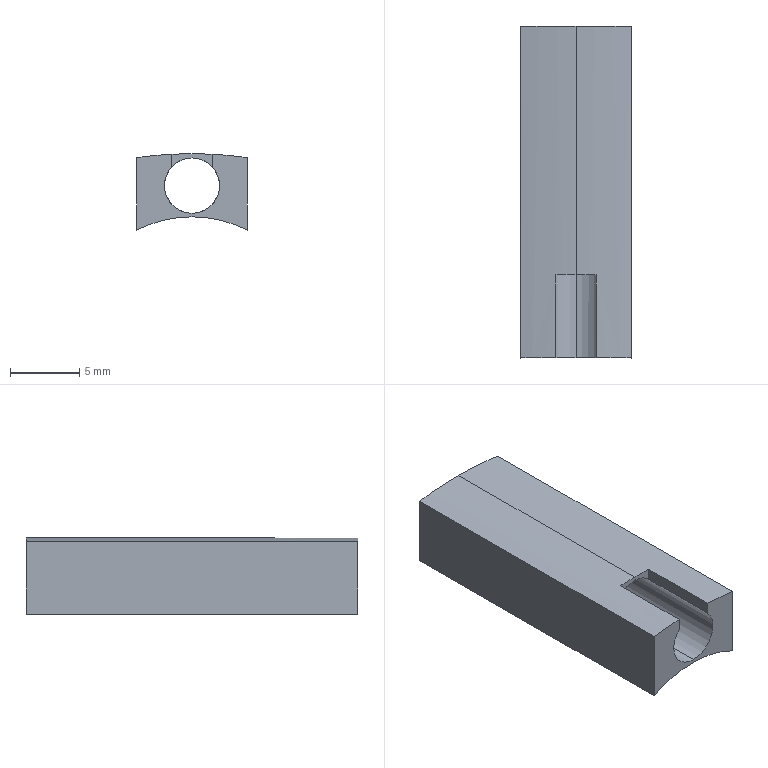Part | NX | 1 solid | 13 faces | box 8 x 24 x 5.527 mm | volume 608.204 mm3 | plane 7 | cylinder 6 | commonest cylinder face diameters 4 x2 17.5 x2 58 x2
STEP:
#1=CARTESIAN_POINT('',(0.,12.,-1.4));
#2=VERTEX_POINT('',#1);
#3=CARTESIAN_POINT('',(0.,12.,2.6));
#4=VERTEX_POINT('',#3);
#5=CARTESIAN_POINT('',(0.,12.,0.6));
#6=DIRECTION('',(0.,1.,0.));
#7=DIRECTION('',(0.,0.,1.));
#8=AXIS2_PLACEMENT_3D('',#5,#6,#7);
#9=CIRCLE('',#8,2.);
#10=EDGE_CURVE('',#2,#4,#9,.T.);
#11=ORIENTED_EDGE('',*,*,#10,.T.);
#12=CARTESIAN_POINT('',(0.,-6.,2.6));
#13=VERTEX_POINT('',#12);
#14=CARTESIAN_POINT('',(0.,-12.,2.6));
#15=DIRECTION('',(0.,1.,0.));
#16=VECTOR('',#15,1000.);
#17=LINE('',#14,#16);
#18=EDGE_CURVE('',#13,#4,#17,.T.);
#19=ORIENTED_EDGE('',*,*,#18,.F.);
#20=CARTESIAN_POINT('',(-1.45,-6.,1.977));
#21=VERTEX_POINT('',#20);
#22=CARTESIAN_POINT('',(0.,-6.,0.6));
#23=DIRECTION('',(0.,1.,0.));
#24=DIRECTION('',(0.,0.,-1.));
#25=AXIS2_PLACEMENT_3D('',#22,#23,#24);
#26=CIRCLE('',#25,2.);
#27=EDGE_CURVE('',#21,#13,#26,.T.);
#28=ORIENTED_EDGE('',*,*,#27,.F.);
#29=CARTESIAN_POINT('',(-1.45,-12.,1.977));
#30=VERTEX_POINT('',#29);
#31=CARTESIAN_POINT('',(-1.45,-6.,1.977));
#32=DIRECTION('',(0.,-1.,0.));
#33=VECTOR('',#32,1000.);
#34=LINE('',#31,#33);
#35=EDGE_CURVE('',#21,#30,#34,.T.);
#36=ORIENTED_EDGE('',*,*,#35,.T.);
#37=CARTESIAN_POINT('',(0.,-12.,-1.4));
#38=VERTEX_POINT('',#37);
#39=CARTESIAN_POINT('',(0.,-12.,0.6));
#40=DIRECTION('',(0.,1.,0.));
#41=DIRECTION('',(0.,0.,1.));
#42=AXIS2_PLACEMENT_3D('',#39,#40,#41);
#43=CIRCLE('',#42,2.);
#44=EDGE_CURVE('',#38,#30,#43,.T.);
#45=ORIENTED_EDGE('',*,*,#44,.F.);
#46=CARTESIAN_POINT('',(0.,-12.,-1.4));
#47=DIRECTION('',(0.,1.,0.));
#48=VECTOR('',#47,1000.);
#49=LINE('',#46,#48);
#50=EDGE_CURVE('',#38,#2,#49,.T.);
#51=ORIENTED_EDGE('',*,*,#50,.T.);
#52=EDGE_LOOP('',(#11,#19,#28,#36,#45,#51));
#53=FACE_BOUND('',#52,.T.);
#54=CARTESIAN_POINT('',(0.,-12.,0.6));
#55=DIRECTION('',(0.,1.,0.));
#56=DIRECTION('',(0.,0.,1.));
#57=AXIS2_PLACEMENT_3D('',#54,#55,#56);
#58=CYLINDRICAL_SURFACE('',#57,2.);
#59=ADVANCED_FACE('',(#53),#58,.F.);
#60=CARTESIAN_POINT('',(0.,-12.,-1.657));
#61=VERTEX_POINT('',#60);
#62=CARTESIAN_POINT('',(0.,12.,-1.657));
#63=VERTEX_POINT('',#62);
#64=CARTESIAN_POINT('',(0.,-12.,-1.657));
#65=DIRECTION('',(0.,1.,0.));
#66=VECTOR('',#65,1000.);
#67=LINE('',#64,#66);
#68=EDGE_CURVE('',#61,#63,#67,.T.);
#69=ORIENTED_EDGE('',*,*,#68,.F.);
#70=CARTESIAN_POINT('',(-4.,-12.,-2.625));
#71=VERTEX_POINT('',#70);
#72=CARTESIAN_POINT('',(0.,-12.,-10.407));
#73=DIRECTION('',(0.,-1.,0.));
#74=DIRECTION('',(0.,0.,1.));
#75=AXIS2_PLACEMENT_3D('',#72,#73,#74);
#76=CIRCLE('',#75,8.75);
#77=EDGE_CURVE('',#61,#71,#76,.T.);
#78=ORIENTED_EDGE('',*,*,#77,.T.);
#79=CARTESIAN_POINT('',(-4.,12.,-2.625));
#80=VERTEX_POINT('',#79);
#81=CARTESIAN_POINT('',(-4.,-12.,-2.625));
#82=DIRECTION('',(0.,1.,0.));
#83=VECTOR('',#82,1000.);
#84=LINE('',#81,#83);
#85=EDGE_CURVE('',#71,#80,#84,.T.);
#86=ORIENTED_EDGE('',*,*,#85,.T.);
#87=CARTESIAN_POINT('',(0.,12.,-10.407));
#88=DIRECTION('',(0.,-1.,0.));
#89=DIRECTION('',(0.,0.,1.));
#90=AXIS2_PLACEMENT_3D('',#87,#88,#89);
#91=CIRCLE('',#90,8.75);
#92=EDGE_CURVE('',#63,#80,#91,.T.);
#93=ORIENTED_EDGE('',*,*,#92,.F.);
#94=EDGE_LOOP('',(#69,#78,#86,#93));
#95=FACE_BOUND('',#94,.T.);
#96=CARTESIAN_POINT('',(0.,-12.,-10.407));
#97=DIRECTION('',(0.,1.,0.));
#98=DIRECTION('',(0.,0.,1.));
#99=AXIS2_PLACEMENT_3D('',#96,#97,#98);
#100=CYLINDRICAL_SURFACE('',#99,8.75);
#101=ADVANCED_FACE('',(#95),#100,.F.);
#102=CARTESIAN_POINT('',(0.,-6.,2.902));
#103=VERTEX_POINT('',#102);
#104=CARTESIAN_POINT('',(0.,12.,2.902));
#105=VERTEX_POINT('',#104);
#106=CARTESIAN_POINT('',(0.,-12.,2.902));
#107=DIRECTION('',(0.,1.,0.));
#108=VECTOR('',#107,1000.);
#109=LINE('',#106,#108);
#110=EDGE_CURVE('',#103,#105,#109,.T.);
#111=ORIENTED_EDGE('',*,*,#110,.F.);
#112=CARTESIAN_POINT('',(1.45,-6.,2.866));
#113=VERTEX_POINT('',#112);
#114=CARTESIAN_POINT('',(0.,-6.,-26.098));
#115=DIRECTION('',(0.,-1.,0.));
#116=DIRECTION('',(0.,0.,-1.));
#117=AXIS2_PLACEMENT_3D('',#114,#115,#116);
#118=CIRCLE('',#117,29.);
#119=EDGE_CURVE('',#113,#103,#118,.T.);
#120=ORIENTED_EDGE('',*,*,#119,.F.);
#121=CARTESIAN_POINT('',(1.45,-12.,2.866));
#122=VERTEX_POINT('',#121);
#123=CARTESIAN_POINT('',(1.45,-6.,2.866));
#124=DIRECTION('',(0.,-1.,0.));
#125=VECTOR('',#124,1000.);
#126=LINE('',#123,#125);
#127=EDGE_CURVE('',#113,#122,#126,.T.);
#128=ORIENTED_EDGE('',*,*,#127,.T.);
#129=CARTESIAN_POINT('',(4.,-12.,2.625));
#130=VERTEX_POINT('',#129);
#131=CARTESIAN_POINT('',(0.,-12.,-26.098));
#132=DIRECTION('',(0.,1.,0.));
#133=DIRECTION('',(0.,0.,-1.));
#134=AXIS2_PLACEMENT_3D('',#131,#132,#133);
#135=CIRCLE('',#134,29.);
#136=EDGE_CURVE('',#122,#130,#135,.T.);
#137=ORIENTED_EDGE('',*,*,#136,.T.);
#138=CARTESIAN_POINT('',(4.,12.,2.625));
#139=VERTEX_POINT('',#138);
#140=CARTESIAN_POINT('',(4.,-12.,2.625));
#141=DIRECTION('',(0.,1.,0.));
#142=VECTOR('',#141,1000.);
#143=LINE('',#140,#142);
#144=EDGE_CURVE('',#130,#139,#143,.T.);
#145=ORIENTED_EDGE('',*,*,#144,.T.);
#146=CARTESIAN_POINT('',(0.,12.,-26.098));
#147=DIRECTION('',(0.,1.,0.));
#148=DIRECTION('',(0.,0.,-1.));
#149=AXIS2_PLACEMENT_3D('',#146,#147,#148);
#150=CIRCLE('',#149,29.);
#151=EDGE_CURVE('',#105,#139,#150,.T.);
#152=ORIENTED_EDGE('',*,*,#151,.F.);
#153=EDGE_LOOP('',(#111,#120,#128,#137,#145,#152));
#154=FACE_BOUND('',#153,.T.);
#155=CARTESIAN_POINT('',(0.,-12.,-26.098));
#156=DIRECTION('',(0.,1.,0.));
#157=DIRECTION('',(0.,0.,1.));
#158=AXIS2_PLACEMENT_3D('',#155,#156,#157);
#159=CYLINDRICAL_SURFACE('',#158,29.);
#160=ADVANCED_FACE('',(#154),#159,.T.);
#161=CARTESIAN_POINT('',(1.45,-12.,1.977));
#162=VERTEX_POINT('',#161);
#163=CARTESIAN_POINT('',(1.45,-12.,1.977));
#164=DIRECTION('',(0.,0.,1.));
#165=VECTOR('',#164,1000.);
#166=LINE('',#163,#165);
#167=EDGE_CURVE('',#162,#122,#166,.T.);
#168=ORIENTED_EDGE('',*,*,#167,.T.);
#169=ORIENTED_EDGE('',*,*,#127,.F.);
#170=CARTESIAN_POINT('',(1.45,-6.,1.977));
#171=VERTEX_POINT('',#170);
#172=CARTESIAN_POINT('',(1.45,-6.,1.977));
#173=DIRECTION('',(0.,0.,1.));
#174=VECTOR('',#173,1000.);
#175=LINE('',#172,#174);
#176=EDGE_CURVE('',#171,#113,#175,.T.);
#177=ORIENTED_EDGE('',*,*,#176,.F.);
#178=CARTESIAN_POINT('',(1.45,-6.,1.977));
#179=DIRECTION('',(0.,-1.,0.));
#180=VECTOR('',#179,1000.);
#181=LINE('',#178,#180);
#182=EDGE_CURVE('',#171,#162,#181,.T.);
#183=ORIENTED_EDGE('',*,*,#182,.T.);
#184=EDGE_LOOP('',(#168,#169,#177,#183));
#185=FACE_BOUND('',#184,.T.);
#186=CARTESIAN_POINT('',(1.45,-6.,1.977));
#187=DIRECTION('',(1.,0.,0.));
#188=DIRECTION('',(0.,1.,0.));
#189=AXIS2_PLACEMENT_3D('',#186,#187,#188);
#190=PLANE('',#189);
#191=ADVANCED_FACE('',(#185),#190,.F.);
#192=CARTESIAN_POINT('',(-4.,12.,2.625));
#193=VERTEX_POINT('',#192);
#194=CARTESIAN_POINT('',(-4.,12.,2.625));
#195=DIRECTION('',(0.,0.,1.));
#196=VECTOR('',#195,1000.);
#197=LINE('',#194,#196);
#198=EDGE_CURVE('',#80,#193,#197,.T.);
#199=ORIENTED_EDGE('',*,*,#198,.F.);
#200=ORIENTED_EDGE('',*,*,#85,.F.);
#201=CARTESIAN_POINT('',(-4.,-12.,2.625));
#202=VERTEX_POINT('',#201);
#203=CARTESIAN_POINT('',(-4.,-12.,2.625));
#204=DIRECTION('',(0.,0.,1.));
#205=VECTOR('',#204,1000.);
#206=LINE('',#203,#205);
#207=EDGE_CURVE('',#71,#202,#206,.T.);
#208=ORIENTED_EDGE('',*,*,#207,.T.);
#209=CARTESIAN_POINT('',(-4.,-12.,2.625));
#210=DIRECTION('',(0.,1.,0.));
#211=VECTOR('',#210,1000.);
#212=LINE('',#209,#211);
#213=EDGE_CURVE('',#202,#193,#212,.T.);
#214=ORIENTED_EDGE('',*,*,#213,.T.);
#215=EDGE_LOOP('',(#199,#200,#208,#214));
#216=FACE_BOUND('',#215,.T.);
#217=CARTESIAN_POINT('',(-4.,-12.,2.625));
#218=DIRECTION('',(-1.,0.,0.));
#219=DIRECTION('',(0.,0.,1.));
#220=AXIS2_PLACEMENT_3D('',#217,#218,#219);
#221=PLANE('',#220);
#222=ADVANCED_FACE('',(#216),#221,.T.);
#223=CARTESIAN_POINT('',(-1.45,-12.,2.866));
#224=VERTEX_POINT('',#223);
#225=CARTESIAN_POINT('',(-1.45,-12.,1.977));
#226=DIRECTION('',(0.,0.,-1.));
#227=VECTOR('',#226,1000.);
#228=LINE('',#225,#227);
#229=EDGE_CURVE('',#224,#30,#228,.T.);
#230=ORIENTED_EDGE('',*,*,#229,.T.);
#231=ORIENTED_EDGE('',*,*,#35,.F.);
#232=CARTESIAN_POINT('',(-1.45,-6.,2.866));
#233=VERTEX_POINT('',#232);
#234=CARTESIAN_POINT('',(-1.45,-6.,1.977));
#235=DIRECTION('',(0.,0.,-1.));
#236=VECTOR('',#235,1000.);
#237=LINE('',#234,#236);
#238=EDGE_CURVE('',#233,#21,#237,.T.);
#239=ORIENTED_EDGE('',*,*,#238,.F.);
#240=CARTESIAN_POINT('',(-1.45,-6.,2.866));
#241=DIRECTION('',(0.,-1.,0.));
#242=VECTOR('',#241,1000.);
#243=LINE('',#240,#242);
#244=EDGE_CURVE('',#233,#224,#243,.T.);
#245=ORIENTED_EDGE('',*,*,#244,.T.);
#246=EDGE_LOOP('',(#230,#231,#239,#245));
#247=FACE_BOUND('',#246,.T.);
#248=CARTESIAN_POINT('',(-1.45,-6.,1.977));
#249=DIRECTION('',(-1.,0.,0.));
#250=DIRECTION('',(0.,0.,1.));
#251=AXIS2_PLACEMENT_3D('',#248,#249,#250);
#252=PLANE('',#251);
#253=ADVANCED_FACE('',(#247),#252,.F.);
#254=CARTESIAN_POINT('',(4.,12.,-2.625));
#255=VERTEX_POINT('',#254);
#256=CARTESIAN_POINT('',(4.,12.,2.625));
#257=DIRECTION('',(0.,0.,-1.));
#258=VECTOR('',#257,1000.);
#259=LINE('',#256,#258);
#260=EDGE_CURVE('',#139,#255,#259,.T.);
#261=ORIENTED_EDGE('',*,*,#260,.F.);
#262=ORIENTED_EDGE('',*,*,#144,.F.);
#263=CARTESIAN_POINT('',(4.,-12.,-2.625));
#264=VERTEX_POINT('',#263);
#265=CARTESIAN_POINT('',(4.,-12.,2.625));
#266=DIRECTION('',(0.,0.,-1.));
#267=VECTOR('',#266,1000.);
#268=LINE('',#265,#267);
#269=EDGE_CURVE('',#130,#264,#268,.T.);
#270=ORIENTED_EDGE('',*,*,#269,.T.);
#271=CARTESIAN_POINT('',(4.,-12.,-2.625));
#272=DIRECTION('',(0.,1.,0.));
#273=VECTOR('',#272,1000.);
#274=LINE('',#271,#273);
#275=EDGE_CURVE('',#264,#255,#274,.T.);
#276=ORIENTED_EDGE('',*,*,#275,.T.);
#277=EDGE_LOOP('',(#261,#262,#270,#276));
#278=FACE_BOUND('',#277,.T.);
#279=CARTESIAN_POINT('',(4.,-12.,2.625));
#280=DIRECTION('',(1.,0.,0.));
#281=DIRECTION('',(0.,1.,0.));
#282=AXIS2_PLACEMENT_3D('',#279,#280,#281);
#283=PLANE('',#282);
#284=ADVANCED_FACE('',(#278),#283,.T.);
#285=ORIENTED_EDGE('',*,*,#229,.F.);
#286=CARTESIAN_POINT('',(0.,-12.,-26.098));
#287=DIRECTION('',(0.,1.,0.));
#288=DIRECTION('',(0.,0.,-1.));
#289=AXIS2_PLACEMENT_3D('',#286,#287,#288);
#290=CIRCLE('',#289,29.);
#291=EDGE_CURVE('',#202,#224,#290,.T.);
#292=ORIENTED_EDGE('',*,*,#291,.F.);
#293=ORIENTED_EDGE('',*,*,#207,.F.);
#294=ORIENTED_EDGE('',*,*,#77,.F.);
#295=CARTESIAN_POINT('',(0.,-12.,-10.407));
#296=DIRECTION('',(0.,-1.,0.));
#297=DIRECTION('',(0.,0.,1.));
#298=AXIS2_PLACEMENT_3D('',#295,#296,#297);
#299=CIRCLE('',#298,8.75);
#300=EDGE_CURVE('',#264,#61,#299,.T.);
#301=ORIENTED_EDGE('',*,*,#300,.F.);
#302=ORIENTED_EDGE('',*,*,#269,.F.);
#303=ORIENTED_EDGE('',*,*,#136,.F.);
#304=ORIENTED_EDGE('',*,*,#167,.F.);
#305=CARTESIAN_POINT('',(0.,-12.,0.6));
#306=DIRECTION('',(0.,1.,0.));
#307=DIRECTION('',(0.,0.,1.));
#308=AXIS2_PLACEMENT_3D('',#305,#306,#307);
#309=CIRCLE('',#308,2.);
#310=EDGE_CURVE('',#162,#38,#309,.T.);
#311=ORIENTED_EDGE('',*,*,#310,.T.);
#312=ORIENTED_EDGE('',*,*,#44,.T.);
#313=EDGE_LOOP('',(#285,#292,#293,#294,#301,#302,#303,#304,#311,#312));
#314=FACE_BOUND('',#313,.T.);
#315=CARTESIAN_POINT('',(0.,-12.,-26.098));
#316=DIRECTION('',(0.,-1.,0.));
#317=DIRECTION('',(0.,0.,-1.));
#318=AXIS2_PLACEMENT_3D('',#315,#316,#317);
#319=PLANE('',#318);
#320=ADVANCED_FACE('',(#314),#319,.T.);
#321=CARTESIAN_POINT('',(0.,12.,-26.098));
#322=DIRECTION('',(0.,1.,0.));
#323=DIRECTION('',(0.,0.,-1.));
#324=AXIS2_PLACEMENT_3D('',#321,#322,#323);
#325=CIRCLE('',#324,29.);
#326=EDGE_CURVE('',#193,#105,#325,.T.);
#327=ORIENTED_EDGE('',*,*,#326,.T.);
#328=ORIENTED_EDGE('',*,*,#151,.T.);
#329=ORIENTED_EDGE('',*,*,#260,.T.);
#330=CARTESIAN_POINT('',(0.,12.,-10.407));
#331=DIRECTION('',(0.,-1.,0.));
#332=DIRECTION('',(0.,0.,1.));
#333=AXIS2_PLACEMENT_3D('',#330,#331,#332);
#334=CIRCLE('',#333,8.75);
#335=EDGE_CURVE('',#255,#63,#334,.T.);
#336=ORIENTED_EDGE('',*,*,#335,.T.);
#337=ORIENTED_EDGE('',*,*,#92,.T.);
#338=ORIENTED_EDGE('',*,*,#198,.T.);
#339=EDGE_LOOP('',(#327,#328,#329,#336,#337,#338));
#340=FACE_BOUND('',#339,.T.);
#341=ORIENTED_EDGE('',*,*,#10,.F.);
#342=CARTESIAN_POINT('',(0.,12.,0.6));
#343=DIRECTION('',(0.,1.,0.));
#344=DIRECTION('',(0.,0.,1.));
#345=AXIS2_PLACEMENT_3D('',#342,#343,#344);
#346=CIRCLE('',#345,2.);
#347=EDGE_CURVE('',#4,#2,#346,.T.);
#348=ORIENTED_EDGE('',*,*,#347,.F.);
#349=EDGE_LOOP('',(#341,#348));
#350=FACE_BOUND('',#349,.T.);
#351=CARTESIAN_POINT('',(0.,12.,-26.098));
#352=DIRECTION('',(0.,-1.,0.));
#353=DIRECTION('',(0.,0.,-1.));
#354=AXIS2_PLACEMENT_3D('',#351,#352,#353);
#355=PLANE('',#354);
#356=ADVANCED_FACE('',(#340,#350),#355,.F.);
#357=CARTESIAN_POINT('',(0.,-6.,0.6));
#358=DIRECTION('',(0.,1.,0.));
#359=DIRECTION('',(0.,0.,-1.));
#360=AXIS2_PLACEMENT_3D('',#357,#358,#359);
#361=CIRCLE('',#360,2.);
#362=EDGE_CURVE('',#13,#171,#361,.T.);
#363=ORIENTED_EDGE('',*,*,#362,.T.);
#364=ORIENTED_EDGE('',*,*,#176,.T.);
#365=ORIENTED_EDGE('',*,*,#119,.T.);
#366=CARTESIAN_POINT('',(0.,-6.,-26.098));
#367=DIRECTION('',(0.,-1.,0.));
#368=DIRECTION('',(0.,0.,-1.));
#369=AXIS2_PLACEMENT_3D('',#366,#367,#368);
#370=CIRCLE('',#369,29.);
#371=EDGE_CURVE('',#103,#233,#370,.T.);
#372=ORIENTED_EDGE('',*,*,#371,.T.);
#373=ORIENTED_EDGE('',*,*,#238,.T.);
#374=ORIENTED_EDGE('',*,*,#27,.T.);
#375=EDGE_LOOP('',(#363,#364,#365,#372,#373,#374));
#376=FACE_BOUND('',#375,.T.);
#377=CARTESIAN_POINT('',(0.,-6.,0.6));
#378=DIRECTION('',(0.,-1.,0.));
#379=DIRECTION('',(0.,0.,-1.));
#380=AXIS2_PLACEMENT_3D('',#377,#378,#379);
#381=PLANE('',#380);
#382=ADVANCED_FACE('',(#376),#381,.T.);
#383=ORIENTED_EDGE('',*,*,#362,.F.);
#384=ORIENTED_EDGE('',*,*,#18,.T.);
#385=ORIENTED_EDGE('',*,*,#347,.T.);
#386=ORIENTED_EDGE('',*,*,#50,.F.);
#387=ORIENTED_EDGE('',*,*,#310,.F.);
#388=ORIENTED_EDGE('',*,*,#182,.F.);
#389=EDGE_LOOP('',(#383,#384,#385,#386,#387,#388));
#390=FACE_BOUND('',#389,.T.);
#391=CARTESIAN_POINT('',(0.,-12.,0.6));
#392=DIRECTION('',(0.,1.,0.));
#393=DIRECTION('',(0.,0.,1.));
#394=AXIS2_PLACEMENT_3D('',#391,#392,#393);
#395=CYLINDRICAL_SURFACE('',#394,2.);
#396=ADVANCED_FACE('',(#390),#395,.F.);
#397=ORIENTED_EDGE('',*,*,#371,.F.);
#398=ORIENTED_EDGE('',*,*,#110,.T.);
#399=ORIENTED_EDGE('',*,*,#326,.F.);
#400=ORIENTED_EDGE('',*,*,#213,.F.);
#401=ORIENTED_EDGE('',*,*,#291,.T.);
#402=ORIENTED_EDGE('',*,*,#244,.F.);
#403=EDGE_LOOP('',(#397,#398,#399,#400,#401,#402));
#404=FACE_BOUND('',#403,.T.);
#405=CARTESIAN_POINT('',(0.,-12.,-26.098));
#406=DIRECTION('',(0.,1.,0.));
#407=DIRECTION('',(0.,0.,1.));
#408=AXIS2_PLACEMENT_3D('',#405,#406,#407);
#409=CYLINDRICAL_SURFACE('',#408,29.);
#410=ADVANCED_FACE('',(#404),#409,.T.);
#411=ORIENTED_EDGE('',*,*,#300,.T.);
#412=ORIENTED_EDGE('',*,*,#68,.T.);
#413=ORIENTED_EDGE('',*,*,#335,.F.);
#414=ORIENTED_EDGE('',*,*,#275,.F.);
#415=EDGE_LOOP('',(#411,#412,#413,#414));
#416=FACE_BOUND('',#415,.T.);
#417=CARTESIAN_POINT('',(0.,-12.,-10.407));
#418=DIRECTION('',(0.,1.,0.));
#419=DIRECTION('',(0.,0.,1.));
#420=AXIS2_PLACEMENT_3D('',#417,#418,#419);
#421=CYLINDRICAL_SURFACE('',#420,8.75);
#422=ADVANCED_FACE('',(#416),#421,.F.);
#423=CLOSED_SHELL('',(#59,#101,#160,#191,#222,#253,#284,#320,#356,#382,#396,#410,#422));
#424=MANIFOLD_SOLID_BREP('',#423);
#425=(LENGTH_UNIT()NAMED_UNIT(*)SI_UNIT(.MILLI.,.METRE.));
#426=UNCERTAINTY_MEASURE_WITH_UNIT(LENGTH_MEASURE(0.00001),#425,'','');
#427=(NAMED_UNIT(*)PLANE_ANGLE_UNIT()SI_UNIT($,.RADIAN.));
#428=(NAMED_UNIT(*)SI_UNIT($,.STERADIAN.)SOLID_ANGLE_UNIT());
#429=(GEOMETRIC_REPRESENTATION_CONTEXT(3)GLOBAL_UNCERTAINTY_ASSIGNED_CONTEXT((#426))GLOBAL_UNIT_ASSIGNED_CONTEXT((#425,#427,#428))REPRESENTATION_CONTEXT('',''));
#430=ADVANCED_BREP_SHAPE_REPRESENTATION('',(#424),#429);